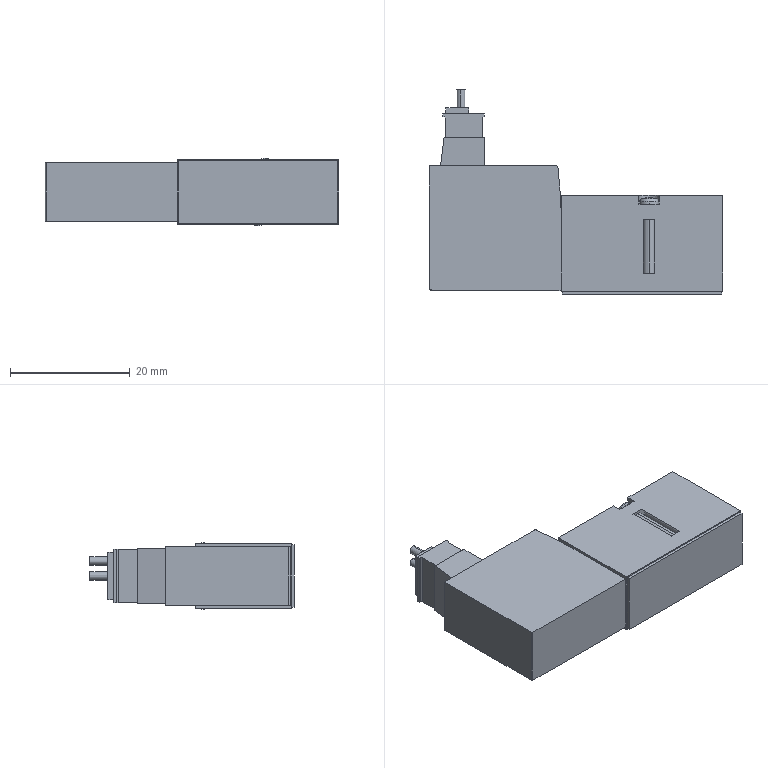Part | SolidWorks | features BaseBody 1 | 1 solid | 106 faces | box 49 x 34.1 x 11.2 mm | volume 9617 mm3 | plane 66 | cylinder 28 | cone 4 | torus 4 | sphere 4 | commonest cylinder face diameters 1 x8 1.4 x4 2 x4 3.4 x4 2.2 x2 3.1 x2